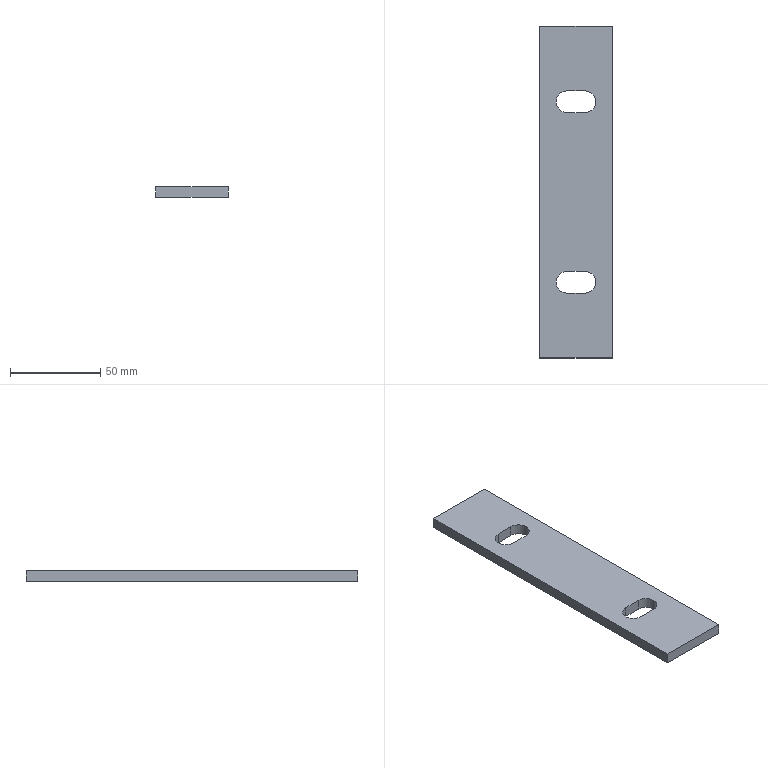Part | STEP file | 护栏连接Plate-200×100 | 1 solid | 16 faces | box 40 x 184 x 6 mm | volume 41363 mm3 | plane 10 | cylinder 6 | commonest cylinder face diameters 12 x6
STEP:
#1=CARTESIAN_POINT('',(0.,0.,0.));
#2=DIRECTION('',(0.,0.,1.));
#3=DIRECTION('',(1.,0.,0.));
#4=AXIS2_PLACEMENT_3D('',#1,#2,#3);
#5=CARTESIAN_POINT('',(5.,56.,0.));
#6=VERTEX_POINT('',#5);
#7=CARTESIAN_POINT('',(5.,56.,6.));
#8=VERTEX_POINT('',#7);
#9=CARTESIAN_POINT('',(5.,56.,6.));
#10=DIRECTION('',(0.,0.,1.));
#11=VECTOR('',#10,1.);
#12=LINE('',#9,#11);
#13=CARTESIAN_POINT('',(5.,50.,6.));
#14=DIRECTION('',(0.,0.,1.));
#15=DIRECTION('',(1.,0.,0.));
#16=AXIS2_PLACEMENT_3D('',#13,#14,#15);
#17=CYLINDRICAL_SURFACE('',#16,6.);
#18=CARTESIAN_POINT('',(1.571,0.));
#19=DIRECTION('',(0.,1.));
#20=VECTOR('',#19,1.);
#21=LINE('',#18,#20);
#22=(GEOMETRIC_REPRESENTATION_CONTEXT(2)PARAMETRIC_REPRESENTATION_CONTEXT()REPRESENTATION_CONTEXT('',''));
#23=DEFINITIONAL_REPRESENTATION('',(#21),#22);
#24=PCURVE('',#17,#23);
#25=CARTESIAN_POINT('',(-5.,56.,6.));
#26=DIRECTION('',(0.,1.,0.));
#27=DIRECTION('',(0.,0.,1.));
#28=AXIS2_PLACEMENT_3D('',#25,#26,#27);
#29=PLANE('',#28);
#30=CARTESIAN_POINT('',(0.,10.));
#31=DIRECTION('',(1.,0.));
#32=VECTOR('',#31,1.);
#33=LINE('',#30,#32);
#34=(GEOMETRIC_REPRESENTATION_CONTEXT(2)PARAMETRIC_REPRESENTATION_CONTEXT()REPRESENTATION_CONTEXT('',''));
#35=DEFINITIONAL_REPRESENTATION('',(#33),#34);
#36=PCURVE('',#29,#35);
#37=SURFACE_CURVE('',#12,(#24,#36),.PCURVE_S1.);
#38=EDGE_CURVE('',#6,#8,#37,.T.);
#39=ORIENTED_EDGE('',*,*,#38,.T.);
#40=CARTESIAN_POINT('',(11.,50.,6.));
#41=VERTEX_POINT('',#40);
#42=CARTESIAN_POINT('',(5.,50.,6.));
#43=DIRECTION('',(0.,0.,1.));
#44=DIRECTION('',(1.,0.,0.));
#45=AXIS2_PLACEMENT_3D('',#42,#43,#44);
#46=CIRCLE('',#45,6.);
#47=CARTESIAN_POINT('',(0.,0.));
#48=DIRECTION('',(1.,0.));
#49=VECTOR('',#48,1.);
#50=LINE('',#47,#49);
#51=(GEOMETRIC_REPRESENTATION_CONTEXT(2)PARAMETRIC_REPRESENTATION_CONTEXT()REPRESENTATION_CONTEXT('',''));
#52=DEFINITIONAL_REPRESENTATION('',(#50),#51);
#53=PCURVE('',#17,#52);
#54=CARTESIAN_POINT('',(0.,0.,6.));
#55=DIRECTION('',(0.,0.,1.));
#56=DIRECTION('',(1.,0.,0.));
#57=AXIS2_PLACEMENT_3D('',#54,#55,#56);
#58=PLANE('',#57);
#59=CARTESIAN_POINT('',(5.,50.));
#60=DIRECTION('',(1.,0.));
#61=AXIS2_PLACEMENT_2D('',#59,#60);
#62=CIRCLE('',#61,6.);
#63=(GEOMETRIC_REPRESENTATION_CONTEXT(2)PARAMETRIC_REPRESENTATION_CONTEXT()REPRESENTATION_CONTEXT('',''));
#64=DEFINITIONAL_REPRESENTATION('',(#62),#63);
#65=PCURVE('',#58,#64);
#66=SURFACE_CURVE('',#46,(#53,#65),.PCURVE_S1.);
#67=EDGE_CURVE('',#41,#8,#66,.T.);
#68=ORIENTED_EDGE('',*,*,#67,.F.);
#69=CARTESIAN_POINT('',(11.,50.,0.));
#70=VERTEX_POINT('',#69);
#71=CARTESIAN_POINT('',(11.,50.,6.));
#72=DIRECTION('',(0.,0.,1.));
#73=VECTOR('',#72,1.);
#74=LINE('',#71,#73);
#75=CARTESIAN_POINT('',(0.,0.));
#76=DIRECTION('',(0.,1.));
#77=VECTOR('',#76,1.);
#78=LINE('',#75,#77);
#79=(GEOMETRIC_REPRESENTATION_CONTEXT(2)PARAMETRIC_REPRESENTATION_CONTEXT()REPRESENTATION_CONTEXT('',''));
#80=DEFINITIONAL_REPRESENTATION('',(#78),#79);
#81=PCURVE('',#17,#80);
#82=CARTESIAN_POINT('',(5.,50.,6.));
#83=DIRECTION('',(0.,0.,1.));
#84=DIRECTION('',(1.,0.,0.));
#85=AXIS2_PLACEMENT_3D('',#82,#83,#84);
#86=CYLINDRICAL_SURFACE('',#85,6.);
#87=CARTESIAN_POINT('',(6.283,0.));
#88=DIRECTION('',(0.,1.));
#89=VECTOR('',#88,1.);
#90=LINE('',#87,#89);
#91=(GEOMETRIC_REPRESENTATION_CONTEXT(2)PARAMETRIC_REPRESENTATION_CONTEXT()REPRESENTATION_CONTEXT('',''));
#92=DEFINITIONAL_REPRESENTATION('',(#90),#91);
#93=PCURVE('',#86,#92);
#94=SURFACE_CURVE('',#74,(#81,#93),.PCURVE_S1.);
#95=EDGE_CURVE('',#70,#41,#94,.T.);
#96=ORIENTED_EDGE('',*,*,#95,.F.);
#97=CARTESIAN_POINT('',(5.,50.,0.));
#98=DIRECTION('',(0.,0.,1.));
#99=DIRECTION('',(1.,0.,0.));
#100=AXIS2_PLACEMENT_3D('',#97,#98,#99);
#101=CIRCLE('',#100,6.);
#102=CARTESIAN_POINT('',(0.,-6.));
#103=DIRECTION('',(1.,0.));
#104=VECTOR('',#103,1.);
#105=LINE('',#102,#104);
#106=(GEOMETRIC_REPRESENTATION_CONTEXT(2)PARAMETRIC_REPRESENTATION_CONTEXT()REPRESENTATION_CONTEXT('',''));
#107=DEFINITIONAL_REPRESENTATION('',(#105),#106);
#108=PCURVE('',#17,#107);
#109=CARTESIAN_POINT('',(0.,0.,0.));
#110=DIRECTION('',(0.,0.,1.));
#111=DIRECTION('',(1.,0.,0.));
#112=AXIS2_PLACEMENT_3D('',#109,#110,#111);
#113=PLANE('',#112);
#114=CARTESIAN_POINT('',(5.,50.));
#115=DIRECTION('',(1.,0.));
#116=AXIS2_PLACEMENT_2D('',#114,#115);
#117=CIRCLE('',#116,6.);
#118=(GEOMETRIC_REPRESENTATION_CONTEXT(2)PARAMETRIC_REPRESENTATION_CONTEXT()REPRESENTATION_CONTEXT('',''));
#119=DEFINITIONAL_REPRESENTATION('',(#117),#118);
#120=PCURVE('',#113,#119);
#121=SURFACE_CURVE('',#101,(#108,#120),.PCURVE_S1.);
#122=EDGE_CURVE('',#70,#6,#121,.T.);
#123=ORIENTED_EDGE('',*,*,#122,.T.);
#124=EDGE_LOOP('',(#39,#68,#96,#123));
#125=FACE_BOUND('',#124,.F.);
#126=ADVANCED_FACE('',(#125),#17,.F.);
#127=CARTESIAN_POINT('',(5.,-44.,0.));
#128=VERTEX_POINT('',#127);
#129=CARTESIAN_POINT('',(5.,-44.,6.));
#130=VERTEX_POINT('',#129);
#131=CARTESIAN_POINT('',(5.,-44.,6.));
#132=DIRECTION('',(0.,0.,1.));
#133=VECTOR('',#132,1.);
#134=LINE('',#131,#133);
#135=CARTESIAN_POINT('',(5.,-50.,6.));
#136=DIRECTION('',(0.,0.,1.));
#137=DIRECTION('',(1.,0.,0.));
#138=AXIS2_PLACEMENT_3D('',#135,#136,#137);
#139=CYLINDRICAL_SURFACE('',#138,6.);
#140=CARTESIAN_POINT('',(1.571,0.));
#141=DIRECTION('',(0.,1.));
#142=VECTOR('',#141,1.);
#143=LINE('',#140,#142);
#144=(GEOMETRIC_REPRESENTATION_CONTEXT(2)PARAMETRIC_REPRESENTATION_CONTEXT()REPRESENTATION_CONTEXT('',''));
#145=DEFINITIONAL_REPRESENTATION('',(#143),#144);
#146=PCURVE('',#139,#145);
#147=CARTESIAN_POINT('',(-5.,-44.,6.));
#148=DIRECTION('',(0.,1.,0.));
#149=DIRECTION('',(0.,0.,1.));
#150=AXIS2_PLACEMENT_3D('',#147,#148,#149);
#151=PLANE('',#150);
#152=CARTESIAN_POINT('',(0.,10.));
#153=DIRECTION('',(1.,0.));
#154=VECTOR('',#153,1.);
#155=LINE('',#152,#154);
#156=(GEOMETRIC_REPRESENTATION_CONTEXT(2)PARAMETRIC_REPRESENTATION_CONTEXT()REPRESENTATION_CONTEXT('',''));
#157=DEFINITIONAL_REPRESENTATION('',(#155),#156);
#158=PCURVE('',#151,#157);
#159=SURFACE_CURVE('',#134,(#146,#158),.PCURVE_S1.);
#160=EDGE_CURVE('',#128,#130,#159,.T.);
#161=ORIENTED_EDGE('',*,*,#160,.T.);
#162=CARTESIAN_POINT('',(11.,-50.,6.));
#163=VERTEX_POINT('',#162);
#164=CARTESIAN_POINT('',(5.,-50.,6.));
#165=DIRECTION('',(0.,0.,1.));
#166=DIRECTION('',(1.,0.,0.));
#167=AXIS2_PLACEMENT_3D('',#164,#165,#166);
#168=CIRCLE('',#167,6.);
#169=CARTESIAN_POINT('',(0.,0.));
#170=DIRECTION('',(1.,0.));
#171=VECTOR('',#170,1.);
#172=LINE('',#169,#171);
#173=(GEOMETRIC_REPRESENTATION_CONTEXT(2)PARAMETRIC_REPRESENTATION_CONTEXT()REPRESENTATION_CONTEXT('',''));
#174=DEFINITIONAL_REPRESENTATION('',(#172),#173);
#175=PCURVE('',#139,#174);
#176=CARTESIAN_POINT('',(5.,-50.));
#177=DIRECTION('',(1.,0.));
#178=AXIS2_PLACEMENT_2D('',#176,#177);
#179=CIRCLE('',#178,6.);
#180=(GEOMETRIC_REPRESENTATION_CONTEXT(2)PARAMETRIC_REPRESENTATION_CONTEXT()REPRESENTATION_CONTEXT('',''));
#181=DEFINITIONAL_REPRESENTATION('',(#179),#180);
#182=PCURVE('',#58,#181);
#183=SURFACE_CURVE('',#168,(#175,#182),.PCURVE_S1.);
#184=EDGE_CURVE('',#163,#130,#183,.T.);
#185=ORIENTED_EDGE('',*,*,#184,.F.);
#186=CARTESIAN_POINT('',(11.,-50.,0.));
#187=VERTEX_POINT('',#186);
#188=CARTESIAN_POINT('',(11.,-50.,6.));
#189=DIRECTION('',(0.,0.,1.));
#190=VECTOR('',#189,1.);
#191=LINE('',#188,#190);
#192=CARTESIAN_POINT('',(0.,0.));
#193=DIRECTION('',(0.,1.));
#194=VECTOR('',#193,1.);
#195=LINE('',#192,#194);
#196=(GEOMETRIC_REPRESENTATION_CONTEXT(2)PARAMETRIC_REPRESENTATION_CONTEXT()REPRESENTATION_CONTEXT('',''));
#197=DEFINITIONAL_REPRESENTATION('',(#195),#196);
#198=PCURVE('',#139,#197);
#199=CARTESIAN_POINT('',(5.,-50.,6.));
#200=DIRECTION('',(0.,0.,1.));
#201=DIRECTION('',(1.,0.,0.));
#202=AXIS2_PLACEMENT_3D('',#199,#200,#201);
#203=CYLINDRICAL_SURFACE('',#202,6.);
#204=CARTESIAN_POINT('',(6.283,0.));
#205=DIRECTION('',(0.,1.));
#206=VECTOR('',#205,1.);
#207=LINE('',#204,#206);
#208=(GEOMETRIC_REPRESENTATION_CONTEXT(2)PARAMETRIC_REPRESENTATION_CONTEXT()REPRESENTATION_CONTEXT('',''));
#209=DEFINITIONAL_REPRESENTATION('',(#207),#208);
#210=PCURVE('',#203,#209);
#211=SURFACE_CURVE('',#191,(#198,#210),.PCURVE_S1.);
#212=EDGE_CURVE('',#187,#163,#211,.T.);
#213=ORIENTED_EDGE('',*,*,#212,.F.);
#214=CARTESIAN_POINT('',(5.,-50.,0.));
#215=DIRECTION('',(0.,0.,1.));
#216=DIRECTION('',(1.,0.,0.));
#217=AXIS2_PLACEMENT_3D('',#214,#215,#216);
#218=CIRCLE('',#217,6.);
#219=CARTESIAN_POINT('',(0.,-6.));
#220=DIRECTION('',(1.,0.));
#221=VECTOR('',#220,1.);
#222=LINE('',#219,#221);
#223=(GEOMETRIC_REPRESENTATION_CONTEXT(2)PARAMETRIC_REPRESENTATION_CONTEXT()REPRESENTATION_CONTEXT('',''));
#224=DEFINITIONAL_REPRESENTATION('',(#222),#223);
#225=PCURVE('',#139,#224);
#226=CARTESIAN_POINT('',(5.,-50.));
#227=DIRECTION('',(1.,0.));
#228=AXIS2_PLACEMENT_2D('',#226,#227);
#229=CIRCLE('',#228,6.);
#230=(GEOMETRIC_REPRESENTATION_CONTEXT(2)PARAMETRIC_REPRESENTATION_CONTEXT()REPRESENTATION_CONTEXT('',''));
#231=DEFINITIONAL_REPRESENTATION('',(#229),#230);
#232=PCURVE('',#113,#231);
#233=SURFACE_CURVE('',#218,(#225,#232),.PCURVE_S1.);
#234=EDGE_CURVE('',#187,#128,#233,.T.);
#235=ORIENTED_EDGE('',*,*,#234,.T.);
#236=EDGE_LOOP('',(#161,#185,#213,#235));
#237=FACE_BOUND('',#236,.F.);
#238=ADVANCED_FACE('',(#237),#139,.F.);
#239=CARTESIAN_POINT('',(20.,-92.,0.));
#240=VERTEX_POINT('',#239);
#241=CARTESIAN_POINT('',(20.,92.,0.));
#242=VERTEX_POINT('',#241);
#243=CARTESIAN_POINT('',(20.,92.,0.));
#244=DIRECTION('',(0.,1.,0.));
#245=VECTOR('',#244,1.);
#246=LINE('',#243,#245);
#247=CARTESIAN_POINT('',(20.,92.,6.));
#248=DIRECTION('',(-1.,0.,0.));
#249=DIRECTION('',(0.,-1.,0.));
#250=AXIS2_PLACEMENT_3D('',#247,#248,#249);
#251=PLANE('',#250);
#252=CARTESIAN_POINT('',(0.,-6.));
#253=DIRECTION('',(-1.,0.));
#254=VECTOR('',#253,1.);
#255=LINE('',#252,#254);
#256=(GEOMETRIC_REPRESENTATION_CONTEXT(2)PARAMETRIC_REPRESENTATION_CONTEXT()REPRESENTATION_CONTEXT('',''));
#257=DEFINITIONAL_REPRESENTATION('',(#255),#256);
#258=PCURVE('',#251,#257);
#259=CARTESIAN_POINT('',(20.,92.));
#260=DIRECTION('',(0.,1.));
#261=VECTOR('',#260,1.);
#262=LINE('',#259,#261);
#263=(GEOMETRIC_REPRESENTATION_CONTEXT(2)PARAMETRIC_REPRESENTATION_CONTEXT()REPRESENTATION_CONTEXT('',''));
#264=DEFINITIONAL_REPRESENTATION('',(#262),#263);
#265=PCURVE('',#113,#264);
#266=SURFACE_CURVE('',#246,(#258,#265),.PCURVE_S1.);
#267=EDGE_CURVE('',#240,#242,#266,.T.);
#268=ORIENTED_EDGE('',*,*,#267,.T.);
#269=CARTESIAN_POINT('',(20.,92.,6.));
#270=VERTEX_POINT('',#269);
#271=CARTESIAN_POINT('',(20.,92.,6.));
#272=DIRECTION('',(0.,0.,-1.));
#273=VECTOR('',#272,1.);
#274=LINE('',#271,#273);
#275=CARTESIAN_POINT('',(0.,0.));
#276=DIRECTION('',(0.,-1.));
#277=VECTOR('',#276,1.);
#278=LINE('',#275,#277);
#279=(GEOMETRIC_REPRESENTATION_CONTEXT(2)PARAMETRIC_REPRESENTATION_CONTEXT()REPRESENTATION_CONTEXT('',''));
#280=DEFINITIONAL_REPRESENTATION('',(#278),#279);
#281=PCURVE('',#251,#280);
#282=CARTESIAN_POINT('',(-20.,92.,6.));
#283=DIRECTION('',(0.,-1.,0.));
#284=DIRECTION('',(0.,0.,-1.));
#285=AXIS2_PLACEMENT_3D('',#282,#283,#284);
#286=PLANE('',#285);
#287=CARTESIAN_POINT('',(0.,40.));
#288=DIRECTION('',(1.,0.));
#289=VECTOR('',#288,1.);
#290=LINE('',#287,#289);
#291=(GEOMETRIC_REPRESENTATION_CONTEXT(2)PARAMETRIC_REPRESENTATION_CONTEXT()REPRESENTATION_CONTEXT('',''));
#292=DEFINITIONAL_REPRESENTATION('',(#290),#291);
#293=PCURVE('',#286,#292);
#294=SURFACE_CURVE('',#274,(#281,#293),.PCURVE_S1.);
#295=EDGE_CURVE('',#270,#242,#294,.T.);
#296=ORIENTED_EDGE('',*,*,#295,.F.);
#297=CARTESIAN_POINT('',(20.,-92.,6.));
#298=VERTEX_POINT('',#297);
#299=CARTESIAN_POINT('',(20.,92.,6.));
#300=DIRECTION('',(0.,1.,0.));
#301=VECTOR('',#300,1.);
#302=LINE('',#299,#301);
#303=CARTESIAN_POINT('',(0.,0.));
#304=DIRECTION('',(-1.,0.));
#305=VECTOR('',#304,1.);
#306=LINE('',#303,#305);
#307=(GEOMETRIC_REPRESENTATION_CONTEXT(2)PARAMETRIC_REPRESENTATION_CONTEXT()REPRESENTATION_CONTEXT('',''));
#308=DEFINITIONAL_REPRESENTATION('',(#306),#307);
#309=PCURVE('',#251,#308);
#310=CARTESIAN_POINT('',(20.,92.));
#311=DIRECTION('',(0.,1.));
#312=VECTOR('',#311,1.);
#313=LINE('',#310,#312);
#314=(GEOMETRIC_REPRESENTATION_CONTEXT(2)PARAMETRIC_REPRESENTATION_CONTEXT()REPRESENTATION_CONTEXT('',''));
#315=DEFINITIONAL_REPRESENTATION('',(#313),#314);
#316=PCURVE('',#58,#315);
#317=SURFACE_CURVE('',#302,(#309,#316),.PCURVE_S1.);
#318=EDGE_CURVE('',#298,#270,#317,.T.);
#319=ORIENTED_EDGE('',*,*,#318,.F.);
#320=CARTESIAN_POINT('',(20.,-92.,6.));
#321=DIRECTION('',(0.,0.,-1.));
#322=VECTOR('',#321,1.);
#323=LINE('',#320,#322);
#324=CARTESIAN_POINT('',(184.,0.));
#325=DIRECTION('',(0.,-1.));
#326=VECTOR('',#325,1.);
#327=LINE('',#324,#326);
#328=(GEOMETRIC_REPRESENTATION_CONTEXT(2)PARAMETRIC_REPRESENTATION_CONTEXT()REPRESENTATION_CONTEXT('',''));
#329=DEFINITIONAL_REPRESENTATION('',(#327),#328);
#330=PCURVE('',#251,#329);
#331=CARTESIAN_POINT('',(-20.,-92.,6.));
#332=DIRECTION('',(0.,1.,0.));
#333=DIRECTION('',(0.,0.,1.));
#334=AXIS2_PLACEMENT_3D('',#331,#332,#333);
#335=PLANE('',#334);
#336=CARTESIAN_POINT('',(0.,40.));
#337=DIRECTION('',(-1.,0.));
#338=VECTOR('',#337,1.);
#339=LINE('',#336,#338);
#340=(GEOMETRIC_REPRESENTATION_CONTEXT(2)PARAMETRIC_REPRESENTATION_CONTEXT()REPRESENTATION_CONTEXT('',''));
#341=DEFINITIONAL_REPRESENTATION('',(#339),#340);
#342=PCURVE('',#335,#341);
#343=SURFACE_CURVE('',#323,(#330,#342),.PCURVE_S1.);
#344=EDGE_CURVE('',#298,#240,#343,.T.);
#345=ORIENTED_EDGE('',*,*,#344,.T.);
#346=EDGE_LOOP('',(#268,#296,#319,#345));
#347=FACE_BOUND('',#346,.T.);
#348=ADVANCED_FACE('',(#347),#251,.F.);
#349=CARTESIAN_POINT('',(-20.,92.,0.));
#350=VERTEX_POINT('',#349);
#351=CARTESIAN_POINT('',(-20.,92.,0.));
#352=DIRECTION('',(-1.,0.,0.));
#353=VECTOR('',#352,1.);
#354=LINE('',#351,#353);
#355=CARTESIAN_POINT('',(6.,0.));
#356=DIRECTION('',(0.,-1.));
#357=VECTOR('',#356,1.);
#358=LINE('',#355,#357);
#359=(GEOMETRIC_REPRESENTATION_CONTEXT(2)PARAMETRIC_REPRESENTATION_CONTEXT()REPRESENTATION_CONTEXT('',''));
#360=DEFINITIONAL_REPRESENTATION('',(#358),#359);
#361=PCURVE('',#286,#360);
#362=CARTESIAN_POINT('',(-20.,92.));
#363=DIRECTION('',(-1.,0.));
#364=VECTOR('',#363,1.);
#365=LINE('',#362,#364);
#366=(GEOMETRIC_REPRESENTATION_CONTEXT(2)PARAMETRIC_REPRESENTATION_CONTEXT()REPRESENTATION_CONTEXT('',''));
#367=DEFINITIONAL_REPRESENTATION('',(#365),#366);
#368=PCURVE('',#113,#367);
#369=SURFACE_CURVE('',#354,(#361,#368),.PCURVE_S1.);
#370=EDGE_CURVE('',#242,#350,#369,.T.);
#371=ORIENTED_EDGE('',*,*,#370,.T.);
#372=CARTESIAN_POINT('',(-20.,92.,6.));
#373=VERTEX_POINT('',#372);
#374=CARTESIAN_POINT('',(-20.,92.,6.));
#375=DIRECTION('',(0.,0.,-1.));
#376=VECTOR('',#375,1.);
#377=LINE('',#374,#376);
#378=CARTESIAN_POINT('',(0.,0.));
#379=DIRECTION('',(1.,0.));
#380=VECTOR('',#379,1.);
#381=LINE('',#378,#380);
#382=(GEOMETRIC_REPRESENTATION_CONTEXT(2)PARAMETRIC_REPRESENTATION_CONTEXT()REPRESENTATION_CONTEXT('',''));
#383=DEFINITIONAL_REPRESENTATION('',(#381),#382);
#384=PCURVE('',#286,#383);
#385=CARTESIAN_POINT('',(-20.,92.,6.));
#386=DIRECTION('',(1.,0.,0.));
#387=DIRECTION('',(0.,1.,0.));
#388=AXIS2_PLACEMENT_3D('',#385,#386,#387);
#389=PLANE('',#388);
#390=CARTESIAN_POINT('',(0.,0.));
#391=DIRECTION('',(0.,-1.));
#392=VECTOR('',#391,1.);
#393=LINE('',#390,#392);
#394=(GEOMETRIC_REPRESENTATION_CONTEXT(2)PARAMETRIC_REPRESENTATION_CONTEXT()REPRESENTATION_CONTEXT('',''));
#395=DEFINITIONAL_REPRESENTATION('',(#393),#394);
#396=PCURVE('',#389,#395);
#397=SURFACE_CURVE('',#377,(#384,#396),.PCURVE_S1.);
#398=EDGE_CURVE('',#373,#350,#397,.T.);
#399=ORIENTED_EDGE('',*,*,#398,.F.);
#400=CARTESIAN_POINT('',(-20.,92.,6.));
#401=DIRECTION('',(-1.,0.,0.));
#402=VECTOR('',#401,1.);
#403=LINE('',#400,#402);
#404=CARTESIAN_POINT('',(0.,0.));
#405=DIRECTION('',(0.,-1.));
#406=VECTOR('',#405,1.);
#407=LINE('',#404,#406);
#408=(GEOMETRIC_REPRESENTATION_CONTEXT(2)PARAMETRIC_REPRESENTATION_CONTEXT()REPRESENTATION_CONTEXT('',''));
#409=DEFINITIONAL_REPRESENTATION('',(#407),#408);
#410=PCURVE('',#286,#409);
#411=CARTESIAN_POINT('',(-20.,92.));
#412=DIRECTION('',(-1.,0.));
#413=VECTOR('',#412,1.);
#414=LINE('',#411,#413);
#415=(GEOMETRIC_REPRESENTATION_CONTEXT(2)PARAMETRIC_REPRESENTATION_CONTEXT()REPRESENTATION_CONTEXT('',''));
#416=DEFINITIONAL_REPRESENTATION('',(#414),#415);
#417=PCURVE('',#58,#416);
#418=SURFACE_CURVE('',#403,(#410,#417),.PCURVE_S1.);
#419=EDGE_CURVE('',#270,#373,#418,.T.);
#420=ORIENTED_EDGE('',*,*,#419,.F.);
#421=ORIENTED_EDGE('',*,*,#295,.T.);
#422=EDGE_LOOP('',(#371,#399,#420,#421));
#423=FACE_BOUND('',#422,.T.);
#424=ADVANCED_FACE('',(#423),#286,.F.);
#425=CARTESIAN_POINT('',(-20.,-92.,0.));
#426=VERTEX_POINT('',#425);
#427=CARTESIAN_POINT('',(-20.,92.,0.));
#428=DIRECTION('',(0.,-1.,0.));
#429=VECTOR('',#428,1.);
#430=LINE('',#427,#429);
#431=CARTESIAN_POINT('',(0.,-6.));
#432=DIRECTION('',(-1.,0.));
#433=VECTOR('',#432,1.);
#434=LINE('',#431,#433);
#435=(GEOMETRIC_REPRESENTATION_CONTEXT(2)PARAMETRIC_REPRESENTATION_CONTEXT()REPRESENTATION_CONTEXT('',''));
#436=DEFINITIONAL_REPRESENTATION('',(#434),#435);
#437=PCURVE('',#389,#436);
#438=CARTESIAN_POINT('',(-20.,92.));
#439=DIRECTION('',(0.,-1.));
#440=VECTOR('',#439,1.);
#441=LINE('',#438,#440);
#442=(GEOMETRIC_REPRESENTATION_CONTEXT(2)PARAMETRIC_REPRESENTATION_CONTEXT()REPRESENTATION_CONTEXT('',''));
#443=DEFINITIONAL_REPRESENTATION('',(#441),#442);
#444=PCURVE('',#113,#443);
#445=SURFACE_CURVE('',#430,(#437,#444),.PCURVE_S1.);
#446=EDGE_CURVE('',#350,#426,#445,.T.);
#447=ORIENTED_EDGE('',*,*,#446,.T.);
#448=CARTESIAN_POINT('',(-20.,-92.,6.));
#449=VERTEX_POINT('',#448);
#450=CARTESIAN_POINT('',(-20.,-92.,6.));
#451=DIRECTION('',(0.,0.,-1.));
#452=VECTOR('',#451,1.);
#453=LINE('',#450,#452);
#454=CARTESIAN_POINT('',(-184.,0.));
#455=DIRECTION('',(0.,-1.));
#456=VECTOR('',#455,1.);
#457=LINE('',#454,#456);
#458=(GEOMETRIC_REPRESENTATION_CONTEXT(2)PARAMETRIC_REPRESENTATION_CONTEXT()REPRESENTATION_CONTEXT('',''));
#459=DEFINITIONAL_REPRESENTATION('',(#457),#458);
#460=PCURVE('',#389,#459);
#461=CARTESIAN_POINT('',(0.,0.));
#462=DIRECTION('',(-1.,0.));
#463=VECTOR('',#462,1.);
#464=LINE('',#461,#463);
#465=(GEOMETRIC_REPRESENTATION_CONTEXT(2)PARAMETRIC_REPRESENTATION_CONTEXT()REPRESENTATION_CONTEXT('',''));
#466=DEFINITIONAL_REPRESENTATION('',(#464),#465);
#467=PCURVE('',#335,#466);
#468=SURFACE_CURVE('',#453,(#460,#467),.PCURVE_S1.);
#469=EDGE_CURVE('',#449,#426,#468,.T.);
#470=ORIENTED_EDGE('',*,*,#469,.F.);
#471=CARTESIAN_POINT('',(-20.,92.,6.));
#472=DIRECTION('',(0.,-1.,0.));
#473=VECTOR('',#472,1.);
#474=LINE('',#471,#473);
#475=CARTESIAN_POINT('',(0.,0.));
#476=DIRECTION('',(-1.,0.));
#477=VECTOR('',#476,1.);
#478=LINE('',#475,#477);
#479=(GEOMETRIC_REPRESENTATION_CONTEXT(2)PARAMETRIC_REPRESENTATION_CONTEXT()REPRESENTATION_CONTEXT('',''));
#480=DEFINITIONAL_REPRESENTATION('',(#478),#479);
#481=PCURVE('',#389,#480);
#482=CARTESIAN_POINT('',(-20.,92.));
#483=DIRECTION('',(0.,-1.));
#484=VECTOR('',#483,1.);
#485=LINE('',#482,#484);
#486=(GEOMETRIC_REPRESENTATION_CONTEXT(2)PARAMETRIC_REPRESENTATION_CONTEXT()REPRESENTATION_CONTEXT('',''));
#487=DEFINITIONAL_REPRESENTATION('',(#485),#486);
#488=PCURVE('',#58,#487);
#489=SURFACE_CURVE('',#474,(#481,#488),.PCURVE_S1.);
#490=EDGE_CURVE('',#373,#449,#489,.T.);
#491=ORIENTED_EDGE('',*,*,#490,.F.);
#492=ORIENTED_EDGE('',*,*,#398,.T.);
#493=EDGE_LOOP('',(#447,#470,#491,#492));
#494=FACE_BOUND('',#493,.T.);
#495=ADVANCED_FACE('',(#494),#389,.F.);
#496=CARTESIAN_POINT('',(-20.,-92.,0.));
#497=DIRECTION('',(1.,0.,0.));
#498=VECTOR('',#497,1.);
#499=LINE('',#496,#498);
#500=CARTESIAN_POINT('',(-6.,0.));
#501=DIRECTION('',(0.,1.));
#502=VECTOR('',#501,1.);
#503=LINE('',#500,#502);
#504=(GEOMETRIC_REPRESENTATION_CONTEXT(2)PARAMETRIC_REPRESENTATION_CONTEXT()REPRESENTATION_CONTEXT('',''));
#505=DEFINITIONAL_REPRESENTATION('',(#503),#504);
#506=PCURVE('',#335,#505);
#507=CARTESIAN_POINT('',(-20.,-92.));
#508=DIRECTION('',(1.,0.));
#509=VECTOR('',#508,1.);
#510=LINE('',#507,#509);
#511=(GEOMETRIC_REPRESENTATION_CONTEXT(2)PARAMETRIC_REPRESENTATION_CONTEXT()REPRESENTATION_CONTEXT('',''));
#512=DEFINITIONAL_REPRESENTATION('',(#510),#511);
#513=PCURVE('',#113,#512);
#514=SURFACE_CURVE('',#499,(#506,#513),.PCURVE_S1.);
#515=EDGE_CURVE('',#426,#240,#514,.T.);
#516=ORIENTED_EDGE('',*,*,#515,.T.);
#517=ORIENTED_EDGE('',*,*,#344,.F.);
#518=CARTESIAN_POINT('',(-20.,-92.,6.));
#519=DIRECTION('',(1.,0.,0.));
#520=VECTOR('',#519,1.);
#521=LINE('',#518,#520);
#522=CARTESIAN_POINT('',(0.,0.));
#523=DIRECTION('',(0.,1.));
#524=VECTOR('',#523,1.);
#525=LINE('',#522,#524);
#526=(GEOMETRIC_REPRESENTATION_CONTEXT(2)PARAMETRIC_REPRESENTATION_CONTEXT()REPRESENTATION_CONTEXT('',''));
#527=DEFINITIONAL_REPRESENTATION('',(#525),#526);
#528=PCURVE('',#335,#527);
#529=CARTESIAN_POINT('',(-20.,-92.));
#530=DIRECTION('',(1.,0.));
#531=VECTOR('',#530,1.);
#532=LINE('',#529,#531);
#533=(GEOMETRIC_REPRESENTATION_CONTEXT(2)PARAMETRIC_REPRESENTATION_CONTEXT()REPRESENTATION_CONTEXT('',''));
#534=DEFINITIONAL_REPRESENTATION('',(#532),#533);
#535=PCURVE('',#58,#534);
#536=SURFACE_CURVE('',#521,(#528,#535),.PCURVE_S1.);
#537=EDGE_CURVE('',#449,#298,#536,.T.);
#538=ORIENTED_EDGE('',*,*,#537,.F.);
#539=ORIENTED_EDGE('',*,*,#469,.T.);
#540=EDGE_LOOP('',(#516,#517,#538,#539));
#541=FACE_BOUND('',#540,.T.);
#542=ADVANCED_FACE('',(#541),#335,.F.);
#543=CARTESIAN_POINT('',(-5.,44.,6.));
#544=VERTEX_POINT('',#543);
#545=CARTESIAN_POINT('',(5.,44.,6.));
#546=VERTEX_POINT('',#545);
#547=CARTESIAN_POINT('',(-5.,44.,6.));
#548=DIRECTION('',(1.,0.,0.));
#549=VECTOR('',#548,1.);
#550=LINE('',#547,#549);
#551=CARTESIAN_POINT('',(-5.,44.));
#552=DIRECTION('',(1.,0.));
#553=VECTOR('',#552,1.);
#554=LINE('',#551,#553);
#555=(GEOMETRIC_REPRESENTATION_CONTEXT(2)PARAMETRIC_REPRESENTATION_CONTEXT()REPRESENTATION_CONTEXT('',''));
#556=DEFINITIONAL_REPRESENTATION('',(#554),#555);
#557=PCURVE('',#58,#556);
#558=CARTESIAN_POINT('',(-5.,44.,6.));
#559=DIRECTION('',(0.,-1.,0.));
#560=DIRECTION('',(0.,0.,-1.));
#561=AXIS2_PLACEMENT_3D('',#558,#559,#560);
#562=PLANE('',#561);
#563=CARTESIAN_POINT('',(0.,0.));
#564=DIRECTION('',(0.,1.));
#565=VECTOR('',#564,1.);
#566=LINE('',#563,#565);
#567=(GEOMETRIC_REPRESENTATION_CONTEXT(2)PARAMETRIC_REPRESENTATION_CONTEXT()REPRESENTATION_CONTEXT('',''));
#568=DEFINITIONAL_REPRESENTATION('',(#566),#567);
#569=PCURVE('',#562,#568);
#570=SURFACE_CURVE('',#550,(#557,#569),.PCURVE_S1.);
#571=EDGE_CURVE('',#544,#546,#570,.T.);
#572=ORIENTED_EDGE('',*,*,#571,.F.);
#573=CARTESIAN_POINT('',(-5.,56.,6.));
#574=VERTEX_POINT('',#573);
#575=CARTESIAN_POINT('',(-5.,50.,6.));
#576=DIRECTION('',(0.,0.,1.));
#577=DIRECTION('',(1.,0.,0.));
#578=AXIS2_PLACEMENT_3D('',#575,#576,#577);
#579=CIRCLE('',#578,6.);
#580=CARTESIAN_POINT('',(-5.,50.));
#581=DIRECTION('',(1.,0.));
#582=AXIS2_PLACEMENT_2D('',#580,#581);
#583=CIRCLE('',#582,6.);
#584=(GEOMETRIC_REPRESENTATION_CONTEXT(2)PARAMETRIC_REPRESENTATION_CONTEXT()REPRESENTATION_CONTEXT('',''));
#585=DEFINITIONAL_REPRESENTATION('',(#583),#584);
#586=PCURVE('',#58,#585);
#587=CARTESIAN_POINT('',(-5.,50.,6.));
#588=DIRECTION('',(0.,0.,1.));
#589=DIRECTION('',(1.,0.,0.));
#590=AXIS2_PLACEMENT_3D('',#587,#588,#589);
#591=CYLINDRICAL_SURFACE('',#590,6.);
#592=CARTESIAN_POINT('',(0.,0.));
#593=DIRECTION('',(1.,0.));
#594=VECTOR('',#593,1.);
#595=LINE('',#592,#594);
#596=(GEOMETRIC_REPRESENTATION_CONTEXT(2)PARAMETRIC_REPRESENTATION_CONTEXT()REPRESENTATION_CONTEXT('',''));
#597=DEFINITIONAL_REPRESENTATION('',(#595),#596);
#598=PCURVE('',#591,#597);
#599=SURFACE_CURVE('',#579,(#586,#598),.PCURVE_S1.);
#600=EDGE_CURVE('',#574,#544,#599,.T.);
#601=ORIENTED_EDGE('',*,*,#600,.F.);
#602=CARTESIAN_POINT('',(-5.,56.,6.));
#603=DIRECTION('',(1.,0.,0.));
#604=VECTOR('',#603,1.);
#605=LINE('',#602,#604);
#606=CARTESIAN_POINT('',(-5.,56.));
#607=DIRECTION('',(1.,0.));
#608=VECTOR('',#607,1.);
#609=LINE('',#606,#608);
#610=(GEOMETRIC_REPRESENTATION_CONTEXT(2)PARAMETRIC_REPRESENTATION_CONTEXT()REPRESENTATION_CONTEXT('',''));
#611=DEFINITIONAL_REPRESENTATION('',(#609),#610);
#612=PCURVE('',#58,#611);
#613=CARTESIAN_POINT('',(0.,0.));
#614=DIRECTION('',(0.,1.));
#615=VECTOR('',#614,1.);
#616=LINE('',#613,#615);
#617=(GEOMETRIC_REPRESENTATION_CONTEXT(2)PARAMETRIC_REPRESENTATION_CONTEXT()REPRESENTATION_CONTEXT('',''));
#618=DEFINITIONAL_REPRESENTATION('',(#616),#617);
#619=PCURVE('',#29,#618);
#620=SURFACE_CURVE('',#605,(#612,#619),.PCURVE_S1.);
#621=EDGE_CURVE('',#574,#8,#620,.T.);
#622=ORIENTED_EDGE('',*,*,#621,.T.);
#623=ORIENTED_EDGE('',*,*,#67,.F.);
#624=CARTESIAN_POINT('',(5.,50.,6.));
#625=DIRECTION('',(0.,0.,1.));
#626=DIRECTION('',(1.,0.,0.));
#627=AXIS2_PLACEMENT_3D('',#624,#625,#626);
#628=CIRCLE('',#627,6.);
#629=CARTESIAN_POINT('',(5.,50.));
#630=DIRECTION('',(1.,0.));
#631=AXIS2_PLACEMENT_2D('',#629,#630);
#632=CIRCLE('',#631,6.);
#633=(GEOMETRIC_REPRESENTATION_CONTEXT(2)PARAMETRIC_REPRESENTATION_CONTEXT()REPRESENTATION_CONTEXT('',''));
#634=DEFINITIONAL_REPRESENTATION('',(#632),#633);
#635=PCURVE('',#58,#634);
#636=CARTESIAN_POINT('',(0.,0.));
#637=DIRECTION('',(1.,0.));
#638=VECTOR('',#637,1.);
#639=LINE('',#636,#638);
#640=(GEOMETRIC_REPRESENTATION_CONTEXT(2)PARAMETRIC_REPRESENTATION_CONTEXT()REPRESENTATION_CONTEXT('',''));
#641=DEFINITIONAL_REPRESENTATION('',(#639),#640);
#642=PCURVE('',#86,#641);
#643=SURFACE_CURVE('',#628,(#635,#642),.PCURVE_S1.);
#644=EDGE_CURVE('',#546,#41,#643,.T.);
#645=ORIENTED_EDGE('',*,*,#644,.F.);
#646=EDGE_LOOP('',(#572,#601,#622,#623,#645));
#647=FACE_BOUND('',#646,.T.);
#648=CARTESIAN_POINT('',(-5.,-56.,6.));
#649=VERTEX_POINT('',#648);
#650=CARTESIAN_POINT('',(5.,-56.,6.));
#651=VERTEX_POINT('',#650);
#652=CARTESIAN_POINT('',(-5.,-56.,6.));
#653=DIRECTION('',(1.,0.,0.));
#654=VECTOR('',#653,1.);
#655=LINE('',#652,#654);
#656=CARTESIAN_POINT('',(-5.,-56.));
#657=DIRECTION('',(1.,0.));
#658=VECTOR('',#657,1.);
#659=LINE('',#656,#658);
#660=(GEOMETRIC_REPRESENTATION_CONTEXT(2)PARAMETRIC_REPRESENTATION_CONTEXT()REPRESENTATION_CONTEXT('',''));
#661=DEFINITIONAL_REPRESENTATION('',(#659),#660);
#662=PCURVE('',#58,#661);
#663=CARTESIAN_POINT('',(-5.,-56.,6.));
#664=DIRECTION('',(0.,-1.,0.));
#665=DIRECTION('',(0.,0.,-1.));
#666=AXIS2_PLACEMENT_3D('',#663,#664,#665);
#667=PLANE('',#666);
#668=CARTESIAN_POINT('',(0.,0.));
#669=DIRECTION('',(0.,1.));
#670=VECTOR('',#669,1.);
#671=LINE('',#668,#670);
#672=(GEOMETRIC_REPRESENTATION_CONTEXT(2)PARAMETRIC_REPRESENTATION_CONTEXT()REPRESENTATION_CONTEXT('',''));
#673=DEFINITIONAL_REPRESENTATION('',(#671),#672);
#674=PCURVE('',#667,#673);
#675=SURFACE_CURVE('',#655,(#662,#674),.PCURVE_S1.);
#676=EDGE_CURVE('',#649,#651,#675,.T.);
#677=ORIENTED_EDGE('',*,*,#676,.F.);
#678=CARTESIAN_POINT('',(-5.,-44.,6.));
#679=VERTEX_POINT('',#678);
#680=CARTESIAN_POINT('',(-5.,-50.,6.));
#681=DIRECTION('',(0.,0.,1.));
#682=DIRECTION('',(1.,0.,0.));
#683=AXIS2_PLACEMENT_3D('',#680,#681,#682);
#684=CIRCLE('',#683,6.);
#685=CARTESIAN_POINT('',(-5.,-50.));
#686=DIRECTION('',(1.,0.));
#687=AXIS2_PLACEMENT_2D('',#685,#686);
#688=CIRCLE('',#687,6.);
#689=(GEOMETRIC_REPRESENTATION_CONTEXT(2)PARAMETRIC_REPRESENTATION_CONTEXT()REPRESENTATION_CONTEXT('',''));
#690=DEFINITIONAL_REPRESENTATION('',(#688),#689);
#691=PCURVE('',#58,#690);
#692=CARTESIAN_POINT('',(-5.,-50.,6.));
#693=DIRECTION('',(0.,0.,1.));
#694=DIRECTION('',(1.,0.,0.));
#695=AXIS2_PLACEMENT_3D('',#692,#693,#694);
#696=CYLINDRICAL_SURFACE('',#695,6.);
#697=CARTESIAN_POINT('',(0.,0.));
#698=DIRECTION('',(1.,0.));
#699=VECTOR('',#698,1.);
#700=LINE('',#697,#699);
#701=(GEOMETRIC_REPRESENTATION_CONTEXT(2)PARAMETRIC_REPRESENTATION_CONTEXT()REPRESENTATION_CONTEXT('',''));
#702=DEFINITIONAL_REPRESENTATION('',(#700),#701);
#703=PCURVE('',#696,#702);
#704=SURFACE_CURVE('',#684,(#691,#703),.PCURVE_S1.);
#705=EDGE_CURVE('',#679,#649,#704,.T.);
#706=ORIENTED_EDGE('',*,*,#705,.F.);
#707=CARTESIAN_POINT('',(-5.,-44.,6.));
#708=DIRECTION('',(1.,0.,0.));
#709=VECTOR('',#708,1.);
#710=LINE('',#707,#709);
#711=CARTESIAN_POINT('',(-5.,-44.));
#712=DIRECTION('',(1.,0.));
#713=VECTOR('',#712,1.);
#714=LINE('',#711,#713);
#715=(GEOMETRIC_REPRESENTATION_CONTEXT(2)PARAMETRIC_REPRESENTATION_CONTEXT()REPRESENTATION_CONTEXT('',''));
#716=DEFINITIONAL_REPRESENTATION('',(#714),#715);
#717=PCURVE('',#58,#716);
#718=CARTESIAN_POINT('',(0.,0.));
#719=DIRECTION('',(0.,1.));
#720=VECTOR('',#719,1.);
#721=LINE('',#718,#720);
#722=(GEOMETRIC_REPRESENTATION_CONTEXT(2)PARAMETRIC_REPRESENTATION_CONTEXT()REPRESENTATION_CONTEXT('',''));
#723=DEFINITIONAL_REPRESENTATION('',(#721),#722);
#724=PCURVE('',#151,#723);
#725=SURFACE_CURVE('',#710,(#717,#724),.PCURVE_S1.);
#726=EDGE_CURVE('',#679,#130,#725,.T.);
#727=ORIENTED_EDGE('',*,*,#726,.T.);
#728=ORIENTED_EDGE('',*,*,#184,.F.);
#729=CARTESIAN_POINT('',(5.,-50.,6.));
#730=DIRECTION('',(0.,0.,1.));
#731=DIRECTION('',(1.,0.,0.));
#732=AXIS2_PLACEMENT_3D('',#729,#730,#731);
#733=CIRCLE('',#732,6.);
#734=CARTESIAN_POINT('',(5.,-50.));
#735=DIRECTION('',(1.,0.));
#736=AXIS2_PLACEMENT_2D('',#734,#735);
#737=CIRCLE('',#736,6.);
#738=(GEOMETRIC_REPRESENTATION_CONTEXT(2)PARAMETRIC_REPRESENTATION_CONTEXT()REPRESENTATION_CONTEXT('',''));
#739=DEFINITIONAL_REPRESENTATION('',(#737),#738);
#740=PCURVE('',#58,#739);
#741=CARTESIAN_POINT('',(0.,0.));
#742=DIRECTION('',(1.,0.));
#743=VECTOR('',#742,1.);
#744=LINE('',#741,#743);
#745=(GEOMETRIC_REPRESENTATION_CONTEXT(2)PARAMETRIC_REPRESENTATION_CONTEXT()REPRESENTATION_CONTEXT('',''));
#746=DEFINITIONAL_REPRESENTATION('',(#744),#745);
#747=PCURVE('',#203,#746);
#748=SURFACE_CURVE('',#733,(#740,#747),.PCURVE_S1.);
#749=EDGE_CURVE('',#651,#163,#748,.T.);
#750=ORIENTED_EDGE('',*,*,#749,.F.);
#751=EDGE_LOOP('',(#677,#706,#727,#728,#750));
#752=FACE_BOUND('',#751,.T.);
#753=ORIENTED_EDGE('',*,*,#318,.T.);
#754=ORIENTED_EDGE('',*,*,#419,.T.);
#755=ORIENTED_EDGE('',*,*,#490,.T.);
#756=ORIENTED_EDGE('',*,*,#537,.T.);
#757=EDGE_LOOP('',(#753,#754,#755,#756));
#758=FACE_BOUND('',#757,.T.);
#759=ADVANCED_FACE('',(#647,#752,#758),#58,.T.);
#760=CARTESIAN_POINT('',(-5.,56.,0.));
#761=VERTEX_POINT('',#760);
#762=CARTESIAN_POINT('',(-5.,56.,0.));
#763=DIRECTION('',(1.,0.,0.));
#764=VECTOR('',#763,1.);
#765=LINE('',#762,#764);
#766=CARTESIAN_POINT('',(-5.,56.));
#767=DIRECTION('',(1.,0.));
#768=VECTOR('',#767,1.);
#769=LINE('',#766,#768);
#770=(GEOMETRIC_REPRESENTATION_CONTEXT(2)PARAMETRIC_REPRESENTATION_CONTEXT()REPRESENTATION_CONTEXT('',''));
#771=DEFINITIONAL_REPRESENTATION('',(#769),#770);
#772=PCURVE('',#113,#771);
#773=CARTESIAN_POINT('',(-6.,0.));
#774=DIRECTION('',(0.,1.));
#775=VECTOR('',#774,1.);
#776=LINE('',#773,#775);
#777=(GEOMETRIC_REPRESENTATION_CONTEXT(2)PARAMETRIC_REPRESENTATION_CONTEXT()REPRESENTATION_CONTEXT('',''));
#778=DEFINITIONAL_REPRESENTATION('',(#776),#777);
#779=PCURVE('',#29,#778);
#780=SURFACE_CURVE('',#765,(#772,#779),.PCURVE_S1.);
#781=EDGE_CURVE('',#761,#6,#780,.T.);
#782=ORIENTED_EDGE('',*,*,#781,.F.);
#783=CARTESIAN_POINT('',(-5.,44.,0.));
#784=VERTEX_POINT('',#783);
#785=CARTESIAN_POINT('',(-5.,50.,0.));
#786=DIRECTION('',(0.,0.,1.));
#787=DIRECTION('',(1.,0.,0.));
#788=AXIS2_PLACEMENT_3D('',#785,#786,#787);
#789=CIRCLE('',#788,6.);
#790=CARTESIAN_POINT('',(-5.,50.));
#791=DIRECTION('',(1.,0.));
#792=AXIS2_PLACEMENT_2D('',#790,#791);
#793=CIRCLE('',#792,6.);
#794=(GEOMETRIC_REPRESENTATION_CONTEXT(2)PARAMETRIC_REPRESENTATION_CONTEXT()REPRESENTATION_CONTEXT('',''));
#795=DEFINITIONAL_REPRESENTATION('',(#793),#794);
#796=PCURVE('',#113,#795);
#797=CARTESIAN_POINT('',(0.,-6.));
#798=DIRECTION('',(1.,0.));
#799=VECTOR('',#798,1.);
#800=LINE('',#797,#799);
#801=(GEOMETRIC_REPRESENTATION_CONTEXT(2)PARAMETRIC_REPRESENTATION_CONTEXT()REPRESENTATION_CONTEXT('',''));
#802=DEFINITIONAL_REPRESENTATION('',(#800),#801);
#803=PCURVE('',#591,#802);
#804=SURFACE_CURVE('',#789,(#796,#803),.PCURVE_S1.);
#805=EDGE_CURVE('',#761,#784,#804,.T.);
#806=ORIENTED_EDGE('',*,*,#805,.T.);
#807=CARTESIAN_POINT('',(5.,44.,0.));
#808=VERTEX_POINT('',#807);
#809=CARTESIAN_POINT('',(-5.,44.,0.));
#810=DIRECTION('',(1.,0.,0.));
#811=VECTOR('',#810,1.);
#812=LINE('',#809,#811);
#813=CARTESIAN_POINT('',(-5.,44.));
#814=DIRECTION('',(1.,0.));
#815=VECTOR('',#814,1.);
#816=LINE('',#813,#815);
#817=(GEOMETRIC_REPRESENTATION_CONTEXT(2)PARAMETRIC_REPRESENTATION_CONTEXT()REPRESENTATION_CONTEXT('',''));
#818=DEFINITIONAL_REPRESENTATION('',(#816),#817);
#819=PCURVE('',#113,#818);
#820=CARTESIAN_POINT('',(6.,0.));
#821=DIRECTION('',(0.,1.));
#822=VECTOR('',#821,1.);
#823=LINE('',#820,#822);
#824=(GEOMETRIC_REPRESENTATION_CONTEXT(2)PARAMETRIC_REPRESENTATION_CONTEXT()REPRESENTATION_CONTEXT('',''));
#825=DEFINITIONAL_REPRESENTATION('',(#823),#824);
#826=PCURVE('',#562,#825);
#827=SURFACE_CURVE('',#812,(#819,#826),.PCURVE_S1.);
#828=EDGE_CURVE('',#784,#808,#827,.T.);
#829=ORIENTED_EDGE('',*,*,#828,.T.);
#830=CARTESIAN_POINT('',(5.,50.,0.));
#831=DIRECTION('',(0.,0.,1.));
#832=DIRECTION('',(1.,0.,0.));
#833=AXIS2_PLACEMENT_3D('',#830,#831,#832);
#834=CIRCLE('',#833,6.);
#835=CARTESIAN_POINT('',(5.,50.));
#836=DIRECTION('',(1.,0.));
#837=AXIS2_PLACEMENT_2D('',#835,#836);
#838=CIRCLE('',#837,6.);
#839=(GEOMETRIC_REPRESENTATION_CONTEXT(2)PARAMETRIC_REPRESENTATION_CONTEXT()REPRESENTATION_CONTEXT('',''));
#840=DEFINITIONAL_REPRESENTATION('',(#838),#839);
#841=PCURVE('',#113,#840);
#842=CARTESIAN_POINT('',(0.,-6.));
#843=DIRECTION('',(1.,0.));
#844=VECTOR('',#843,1.);
#845=LINE('',#842,#844);
#846=(GEOMETRIC_REPRESENTATION_CONTEXT(2)PARAMETRIC_REPRESENTATION_CONTEXT()REPRESENTATION_CONTEXT('',''));
#847=DEFINITIONAL_REPRESENTATION('',(#845),#846);
#848=PCURVE('',#86,#847);
#849=SURFACE_CURVE('',#834,(#841,#848),.PCURVE_S1.);
#850=EDGE_CURVE('',#808,#70,#849,.T.);
#851=ORIENTED_EDGE('',*,*,#850,.T.);
#852=ORIENTED_EDGE('',*,*,#122,.T.);
#853=EDGE_LOOP('',(#782,#806,#829,#851,#852));
#854=FACE_BOUND('',#853,.T.);
#855=CARTESIAN_POINT('',(-5.,-56.,0.));
#856=VERTEX_POINT('',#855);
#857=CARTESIAN_POINT('',(5.,-56.,0.));
#858=VERTEX_POINT('',#857);
#859=CARTESIAN_POINT('',(-5.,-56.,0.));
#860=DIRECTION('',(1.,0.,0.));
#861=VECTOR('',#860,1.);
#862=LINE('',#859,#861);
#863=CARTESIAN_POINT('',(-5.,-56.));
#864=DIRECTION('',(1.,0.));
#865=VECTOR('',#864,1.);
#866=LINE('',#863,#865);
#867=(GEOMETRIC_REPRESENTATION_CONTEXT(2)PARAMETRIC_REPRESENTATION_CONTEXT()REPRESENTATION_CONTEXT('',''));
#868=DEFINITIONAL_REPRESENTATION('',(#866),#867);
#869=PCURVE('',#113,#868);
#870=CARTESIAN_POINT('',(6.,0.));
#871=DIRECTION('',(0.,1.));
#872=VECTOR('',#871,1.);
#873=LINE('',#870,#872);
#874=(GEOMETRIC_REPRESENTATION_CONTEXT(2)PARAMETRIC_REPRESENTATION_CONTEXT()REPRESENTATION_CONTEXT('',''));
#875=DEFINITIONAL_REPRESENTATION('',(#873),#874);
#876=PCURVE('',#667,#875);
#877=SURFACE_CURVE('',#862,(#869,#876),.PCURVE_S1.);
#878=EDGE_CURVE('',#856,#858,#877,.T.);
#879=ORIENTED_EDGE('',*,*,#878,.T.);
#880=CARTESIAN_POINT('',(5.,-50.,0.));
#881=DIRECTION('',(0.,0.,1.));
#882=DIRECTION('',(1.,0.,0.));
#883=AXIS2_PLACEMENT_3D('',#880,#881,#882);
#884=CIRCLE('',#883,6.);
#885=CARTESIAN_POINT('',(5.,-50.));
#886=DIRECTION('',(1.,0.));
#887=AXIS2_PLACEMENT_2D('',#885,#886);
#888=CIRCLE('',#887,6.);
#889=(GEOMETRIC_REPRESENTATION_CONTEXT(2)PARAMETRIC_REPRESENTATION_CONTEXT()REPRESENTATION_CONTEXT('',''));
#890=DEFINITIONAL_REPRESENTATION('',(#888),#889);
#891=PCURVE('',#113,#890);
#892=CARTESIAN_POINT('',(0.,-6.));
#893=DIRECTION('',(1.,0.));
#894=VECTOR('',#893,1.);
#895=LINE('',#892,#894);
#896=(GEOMETRIC_REPRESENTATION_CONTEXT(2)PARAMETRIC_REPRESENTATION_CONTEXT()REPRESENTATION_CONTEXT('',''));
#897=DEFINITIONAL_REPRESENTATION('',(#895),#896);
#898=PCURVE('',#203,#897);
#899=SURFACE_CURVE('',#884,(#891,#898),.PCURVE_S1.);
#900=EDGE_CURVE('',#858,#187,#899,.T.);
#901=ORIENTED_EDGE('',*,*,#900,.T.);
#902=ORIENTED_EDGE('',*,*,#234,.T.);
#903=CARTESIAN_POINT('',(-5.,-44.,0.));
#904=VERTEX_POINT('',#903);
#905=CARTESIAN_POINT('',(-5.,-44.,0.));
#906=DIRECTION('',(1.,0.,0.));
#907=VECTOR('',#906,1.);
#908=LINE('',#905,#907);
#909=CARTESIAN_POINT('',(-5.,-44.));
#910=DIRECTION('',(1.,0.));
#911=VECTOR('',#910,1.);
#912=LINE('',#909,#911);
#913=(GEOMETRIC_REPRESENTATION_CONTEXT(2)PARAMETRIC_REPRESENTATION_CONTEXT()REPRESENTATION_CONTEXT('',''));
#914=DEFINITIONAL_REPRESENTATION('',(#912),#913);
#915=PCURVE('',#113,#914);
#916=CARTESIAN_POINT('',(-6.,0.));
#917=DIRECTION('',(0.,1.));
#918=VECTOR('',#917,1.);
#919=LINE('',#916,#918);
#920=(GEOMETRIC_REPRESENTATION_CONTEXT(2)PARAMETRIC_REPRESENTATION_CONTEXT()REPRESENTATION_CONTEXT('',''));
#921=DEFINITIONAL_REPRESENTATION('',(#919),#920);
#922=PCURVE('',#151,#921);
#923=SURFACE_CURVE('',#908,(#915,#922),.PCURVE_S1.);
#924=EDGE_CURVE('',#904,#128,#923,.T.);
#925=ORIENTED_EDGE('',*,*,#924,.F.);
#926=CARTESIAN_POINT('',(-5.,-50.,0.));
#927=DIRECTION('',(0.,0.,1.));
#928=DIRECTION('',(1.,0.,0.));
#929=AXIS2_PLACEMENT_3D('',#926,#927,#928);
#930=CIRCLE('',#929,6.);
#931=CARTESIAN_POINT('',(-5.,-50.));
#932=DIRECTION('',(1.,0.));
#933=AXIS2_PLACEMENT_2D('',#931,#932);
#934=CIRCLE('',#933,6.);
#935=(GEOMETRIC_REPRESENTATION_CONTEXT(2)PARAMETRIC_REPRESENTATION_CONTEXT()REPRESENTATION_CONTEXT('',''));
#936=DEFINITIONAL_REPRESENTATION('',(#934),#935);
#937=PCURVE('',#113,#936);
#938=CARTESIAN_POINT('',(0.,-6.));
#939=DIRECTION('',(1.,0.));
#940=VECTOR('',#939,1.);
#941=LINE('',#938,#940);
#942=(GEOMETRIC_REPRESENTATION_CONTEXT(2)PARAMETRIC_REPRESENTATION_CONTEXT()REPRESENTATION_CONTEXT('',''));
#943=DEFINITIONAL_REPRESENTATION('',(#941),#942);
#944=PCURVE('',#696,#943);
#945=SURFACE_CURVE('',#930,(#937,#944),.PCURVE_S1.);
#946=EDGE_CURVE('',#904,#856,#945,.T.);
#947=ORIENTED_EDGE('',*,*,#946,.T.);
#948=EDGE_LOOP('',(#879,#901,#902,#925,#947));
#949=FACE_BOUND('',#948,.T.);
#950=ORIENTED_EDGE('',*,*,#267,.F.);
#951=ORIENTED_EDGE('',*,*,#515,.F.);
#952=ORIENTED_EDGE('',*,*,#446,.F.);
#953=ORIENTED_EDGE('',*,*,#370,.F.);
#954=EDGE_LOOP('',(#950,#951,#952,#953));
#955=FACE_BOUND('',#954,.T.);
#956=ADVANCED_FACE('',(#854,#949,#955),#113,.F.);
#957=ORIENTED_EDGE('',*,*,#749,.F.);
#958=CARTESIAN_POINT('',(5.,-56.,6.));
#959=DIRECTION('',(0.,0.,-1.));
#960=VECTOR('',#959,1.);
#961=LINE('',#958,#960);
#962=CARTESIAN_POINT('',(4.712,0.));
#963=DIRECTION('',(0.,-1.));
#964=VECTOR('',#963,1.);
#965=LINE('',#962,#964);
#966=(GEOMETRIC_REPRESENTATION_CONTEXT(2)PARAMETRIC_REPRESENTATION_CONTEXT()REPRESENTATION_CONTEXT('',''));
#967=DEFINITIONAL_REPRESENTATION('',(#965),#966);
#968=PCURVE('',#203,#967);
#969=CARTESIAN_POINT('',(0.,10.));
#970=DIRECTION('',(1.,0.));
#971=VECTOR('',#970,1.);
#972=LINE('',#969,#971);
#973=(GEOMETRIC_REPRESENTATION_CONTEXT(2)PARAMETRIC_REPRESENTATION_CONTEXT()REPRESENTATION_CONTEXT('',''));
#974=DEFINITIONAL_REPRESENTATION('',(#972),#973);
#975=PCURVE('',#667,#974);
#976=SURFACE_CURVE('',#961,(#968,#975),.PCURVE_S1.);
#977=EDGE_CURVE('',#651,#858,#976,.T.);
#978=ORIENTED_EDGE('',*,*,#977,.T.);
#979=ORIENTED_EDGE('',*,*,#900,.T.);
#980=ORIENTED_EDGE('',*,*,#212,.T.);
#981=EDGE_LOOP('',(#957,#978,#979,#980));
#982=FACE_BOUND('',#981,.F.);
#983=ADVANCED_FACE('',(#982),#203,.F.);
#984=CARTESIAN_POINT('',(-5.,-44.,6.));
#985=DIRECTION('',(0.,0.,-1.));
#986=VECTOR('',#985,1.);
#987=LINE('',#984,#986);
#988=CARTESIAN_POINT('',(1.571,0.));
#989=DIRECTION('',(0.,-1.));
#990=VECTOR('',#989,1.);
#991=LINE('',#988,#990);
#992=(GEOMETRIC_REPRESENTATION_CONTEXT(2)PARAMETRIC_REPRESENTATION_CONTEXT()REPRESENTATION_CONTEXT('',''));
#993=DEFINITIONAL_REPRESENTATION('',(#991),#992);
#994=PCURVE('',#696,#993);
#995=CARTESIAN_POINT('',(0.,0.));
#996=DIRECTION('',(-1.,0.));
#997=VECTOR('',#996,1.);
#998=LINE('',#995,#997);
#999=(GEOMETRIC_REPRESENTATION_CONTEXT(2)PARAMETRIC_REPRESENTATION_CONTEXT()REPRESENTATION_CONTEXT('',''));
#1000=DEFINITIONAL_REPRESENTATION('',(#998),#999);
#1001=PCURVE('',#151,#1000);
#1002=SURFACE_CURVE('',#987,(#994,#1001),.PCURVE_S1.);
#1003=EDGE_CURVE('',#679,#904,#1002,.T.);
#1004=ORIENTED_EDGE('',*,*,#1003,.T.);
#1005=ORIENTED_EDGE('',*,*,#946,.T.);
#1006=CARTESIAN_POINT('',(-5.,-56.,6.));
#1007=DIRECTION('',(0.,0.,1.));
#1008=VECTOR('',#1007,1.);
#1009=LINE('',#1006,#1008);
#1010=CARTESIAN_POINT('',(4.712,0.));
#1011=DIRECTION('',(0.,1.));
#1012=VECTOR('',#1011,1.);
#1013=LINE('',#1010,#1012);
#1014=(GEOMETRIC_REPRESENTATION_CONTEXT(2)PARAMETRIC_REPRESENTATION_CONTEXT()REPRESENTATION_CONTEXT('',''));
#1015=DEFINITIONAL_REPRESENTATION('',(#1013),#1014);
#1016=PCURVE('',#696,#1015);
#1017=CARTESIAN_POINT('',(0.,0.));
#1018=DIRECTION('',(-1.,0.));
#1019=VECTOR('',#1018,1.);
#1020=LINE('',#1017,#1019);
#1021=(GEOMETRIC_REPRESENTATION_CONTEXT(2)PARAMETRIC_REPRESENTATION_CONTEXT()REPRESENTATION_CONTEXT('',''));
#1022=DEFINITIONAL_REPRESENTATION('',(#1020),#1021);
#1023=PCURVE('',#667,#1022);
#1024=SURFACE_CURVE('',#1009,(#1016,#1023),.PCURVE_S1.);
#1025=EDGE_CURVE('',#856,#649,#1024,.T.);
#1026=ORIENTED_EDGE('',*,*,#1025,.T.);
#1027=ORIENTED_EDGE('',*,*,#705,.F.);
#1028=EDGE_LOOP('',(#1004,#1005,#1026,#1027));
#1029=FACE_BOUND('',#1028,.F.);
#1030=ADVANCED_FACE('',(#1029),#696,.F.);
#1031=ORIENTED_EDGE('',*,*,#160,.T.);
#1032=ORIENTED_EDGE('',*,*,#726,.F.);
#1033=ORIENTED_EDGE('',*,*,#1003,.T.);
#1034=ORIENTED_EDGE('',*,*,#924,.T.);
#1035=EDGE_LOOP('',(#1031,#1032,#1033,#1034));
#1036=FACE_BOUND('',#1035,.T.);
#1037=ADVANCED_FACE('',(#1036),#151,.F.);
#1038=ORIENTED_EDGE('',*,*,#977,.T.);
#1039=ORIENTED_EDGE('',*,*,#878,.F.);
#1040=ORIENTED_EDGE('',*,*,#1025,.T.);
#1041=ORIENTED_EDGE('',*,*,#676,.T.);
#1042=EDGE_LOOP('',(#1038,#1039,#1040,#1041));
#1043=FACE_BOUND('',#1042,.T.);
#1044=ADVANCED_FACE('',(#1043),#667,.F.);
#1045=ORIENTED_EDGE('',*,*,#644,.F.);
#1046=CARTESIAN_POINT('',(5.,44.,6.));
#1047=DIRECTION('',(0.,0.,-1.));
#1048=VECTOR('',#1047,1.);
#1049=LINE('',#1046,#1048);
#1050=CARTESIAN_POINT('',(4.712,0.));
#1051=DIRECTION('',(0.,-1.));
#1052=VECTOR('',#1051,1.);
#1053=LINE('',#1050,#1052);
#1054=(GEOMETRIC_REPRESENTATION_CONTEXT(2)PARAMETRIC_REPRESENTATION_CONTEXT()REPRESENTATION_CONTEXT('',''));
#1055=DEFINITIONAL_REPRESENTATION('',(#1053),#1054);
#1056=PCURVE('',#86,#1055);
#1057=CARTESIAN_POINT('',(0.,10.));
#1058=DIRECTION('',(1.,0.));
#1059=VECTOR('',#1058,1.);
#1060=LINE('',#1057,#1059);
#1061=(GEOMETRIC_REPRESENTATION_CONTEXT(2)PARAMETRIC_REPRESENTATION_CONTEXT()REPRESENTATION_CONTEXT('',''));
#1062=DEFINITIONAL_REPRESENTATION('',(#1060),#1061);
#1063=PCURVE('',#562,#1062);
#1064=SURFACE_CURVE('',#1049,(#1056,#1063),.PCURVE_S1.);
#1065=EDGE_CURVE('',#546,#808,#1064,.T.);
#1066=ORIENTED_EDGE('',*,*,#1065,.T.);
#1067=ORIENTED_EDGE('',*,*,#850,.T.);
#1068=ORIENTED_EDGE('',*,*,#95,.T.);
#1069=EDGE_LOOP('',(#1045,#1066,#1067,#1068));
#1070=FACE_BOUND('',#1069,.F.);
#1071=ADVANCED_FACE('',(#1070),#86,.F.);
#1072=CARTESIAN_POINT('',(-5.,56.,6.));
#1073=DIRECTION('',(0.,0.,-1.));
#1074=VECTOR('',#1073,1.);
#1075=LINE('',#1072,#1074);
#1076=CARTESIAN_POINT('',(1.571,0.));
#1077=DIRECTION('',(0.,-1.));
#1078=VECTOR('',#1077,1.);
#1079=LINE('',#1076,#1078);
#1080=(GEOMETRIC_REPRESENTATION_CONTEXT(2)PARAMETRIC_REPRESENTATION_CONTEXT()REPRESENTATION_CONTEXT('',''));
#1081=DEFINITIONAL_REPRESENTATION('',(#1079),#1080);
#1082=PCURVE('',#591,#1081);
#1083=CARTESIAN_POINT('',(0.,0.));
#1084=DIRECTION('',(-1.,0.));
#1085=VECTOR('',#1084,1.);
#1086=LINE('',#1083,#1085);
#1087=(GEOMETRIC_REPRESENTATION_CONTEXT(2)PARAMETRIC_REPRESENTATION_CONTEXT()REPRESENTATION_CONTEXT('',''));
#1088=DEFINITIONAL_REPRESENTATION('',(#1086),#1087);
#1089=PCURVE('',#29,#1088);
#1090=SURFACE_CURVE('',#1075,(#1082,#1089),.PCURVE_S1.);
#1091=EDGE_CURVE('',#574,#761,#1090,.T.);
#1092=ORIENTED_EDGE('',*,*,#1091,.T.);
#1093=ORIENTED_EDGE('',*,*,#805,.T.);
#1094=CARTESIAN_POINT('',(-5.,44.,6.));
#1095=DIRECTION('',(0.,0.,1.));
#1096=VECTOR('',#1095,1.);
#1097=LINE('',#1094,#1096);
#1098=CARTESIAN_POINT('',(4.712,0.));
#1099=DIRECTION('',(0.,1.));
#1100=VECTOR('',#1099,1.);
#1101=LINE('',#1098,#1100);
#1102=(GEOMETRIC_REPRESENTATION_CONTEXT(2)PARAMETRIC_REPRESENTATION_CONTEXT()REPRESENTATION_CONTEXT('',''));
#1103=DEFINITIONAL_REPRESENTATION('',(#1101),#1102);
#1104=PCURVE('',#591,#1103);
#1105=CARTESIAN_POINT('',(0.,0.));
#1106=DIRECTION('',(-1.,0.));
#1107=VECTOR('',#1106,1.);
#1108=LINE('',#1105,#1107);
#1109=(GEOMETRIC_REPRESENTATION_CONTEXT(2)PARAMETRIC_REPRESENTATION_CONTEXT()REPRESENTATION_CONTEXT('',''));
#1110=DEFINITIONAL_REPRESENTATION('',(#1108),#1109);
#1111=PCURVE('',#562,#1110);
#1112=SURFACE_CURVE('',#1097,(#1104,#1111),.PCURVE_S1.);
#1113=EDGE_CURVE('',#784,#544,#1112,.T.);
#1114=ORIENTED_EDGE('',*,*,#1113,.T.);
#1115=ORIENTED_EDGE('',*,*,#600,.F.);
#1116=EDGE_LOOP('',(#1092,#1093,#1114,#1115));
#1117=FACE_BOUND('',#1116,.F.);
#1118=ADVANCED_FACE('',(#1117),#591,.F.);
#1119=ORIENTED_EDGE('',*,*,#38,.T.);
#1120=ORIENTED_EDGE('',*,*,#621,.F.);
#1121=ORIENTED_EDGE('',*,*,#1091,.T.);
#1122=ORIENTED_EDGE('',*,*,#781,.T.);
#1123=EDGE_LOOP('',(#1119,#1120,#1121,#1122));
#1124=FACE_BOUND('',#1123,.T.);
#1125=ADVANCED_FACE('',(#1124),#29,.F.);
#1126=ORIENTED_EDGE('',*,*,#1065,.T.);
#1127=ORIENTED_EDGE('',*,*,#828,.F.);
#1128=ORIENTED_EDGE('',*,*,#1113,.T.);
#1129=ORIENTED_EDGE('',*,*,#571,.T.);
#1130=EDGE_LOOP('',(#1126,#1127,#1128,#1129));
#1131=FACE_BOUND('',#1130,.T.);
#1132=ADVANCED_FACE('',(#1131),#562,.F.);
#1133=CLOSED_SHELL('',(#126,#238,#348,#424,#495,#542,#759,#956,#983,#1030,#1037,#1044,#1071,#1118,#1125,#1132));
#1134=MANIFOLD_SOLID_BREP('',#1133);
#1135=(LENGTH_UNIT()NAMED_UNIT(*)SI_UNIT(.MILLI.,.METRE.));
#1136=UNCERTAINTY_MEASURE_WITH_UNIT(LENGTH_MEASURE(0.0000001),#1135,'','');
#1137=(NAMED_UNIT(*)PLANE_ANGLE_UNIT()SI_UNIT($,.RADIAN.));
#1138=(NAMED_UNIT(*)SI_UNIT($,.STERADIAN.)SOLID_ANGLE_UNIT());
#1139=(GEOMETRIC_REPRESENTATION_CONTEXT(3)GLOBAL_UNCERTAINTY_ASSIGNED_CONTEXT((#1136))GLOBAL_UNIT_ASSIGNED_CONTEXT((#1135,#1137,#1138))REPRESENTATION_CONTEXT('',''));
#1140=ADVANCED_BREP_SHAPE_REPRESENTATION('',(#4,#1134),#1139);